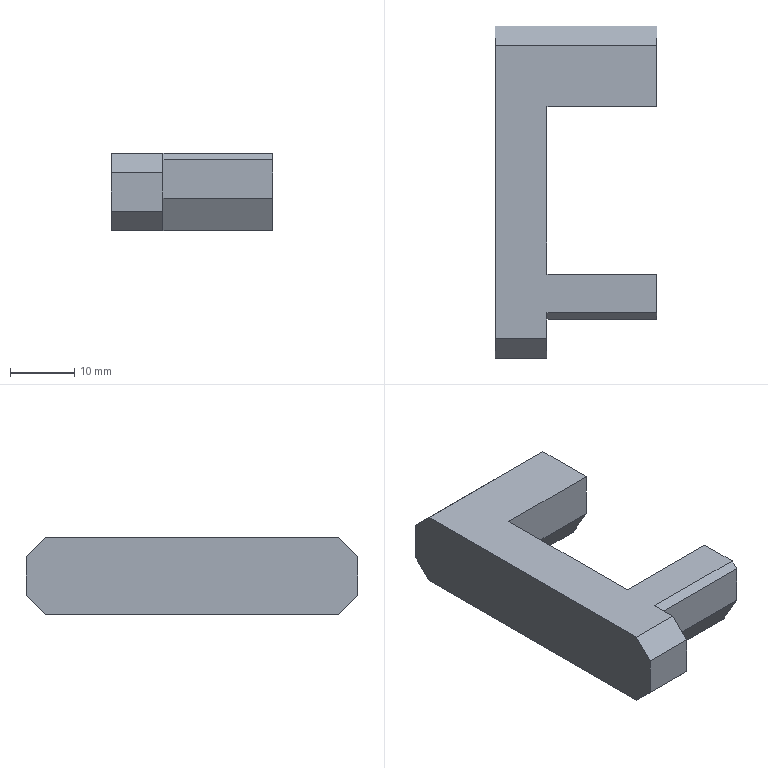Part | NX | features solid 2 | 1 solid | 19 faces | box 25 x 51.5 x 12 mm | volume 8371 mm3 | plane 19
STEP:
#1=CARTESIAN_POINT('',(256.5,-270.,46.5));
#2=VERTEX_POINT('',#1);
#3=CARTESIAN_POINT('',(256.5,-270.,52.5));
#4=VERTEX_POINT('',#3);
#5=CARTESIAN_POINT('',(256.5,-270.,46.5));
#6=DIRECTION('',(0.,0.,1.));
#7=VECTOR('',#6,1000.);
#8=LINE('',#5,#7);
#9=EDGE_CURVE('',#2,#4,#8,.T.);
#10=ORIENTED_EDGE('',*,*,#9,.F.);
#11=CARTESIAN_POINT('',(256.5,-267.113,41.5));
#12=VERTEX_POINT('',#11);
#13=CARTESIAN_POINT('',(256.5,-267.113,41.5));
#14=DIRECTION('',(0.,-0.5,0.866));
#15=VECTOR('',#14,1000.);
#16=LINE('',#13,#15);
#17=EDGE_CURVE('',#12,#2,#16,.T.);
#18=ORIENTED_EDGE('',*,*,#17,.F.);
#19=CARTESIAN_POINT('',(256.5,-263.,41.5));
#20=VERTEX_POINT('',#19);
#21=CARTESIAN_POINT('',(256.5,-263.,41.5));
#22=DIRECTION('',(0.,-1.,0.));
#23=VECTOR('',#22,1000.);
#24=LINE('',#21,#23);
#25=EDGE_CURVE('',#20,#12,#24,.T.);
#26=ORIENTED_EDGE('',*,*,#25,.F.);
#27=CARTESIAN_POINT('',(256.5,-263.,53.5));
#28=VERTEX_POINT('',#27);
#29=CARTESIAN_POINT('',(256.5,-263.,41.5));
#30=DIRECTION('',(0.,0.,1.));
#31=VECTOR('',#30,1000.);
#32=LINE('',#29,#31);
#33=EDGE_CURVE('',#20,#28,#32,.T.);
#34=ORIENTED_EDGE('',*,*,#33,.T.);
#35=CARTESIAN_POINT('',(256.5,-269.,53.5));
#36=VERTEX_POINT('',#35);
#37=CARTESIAN_POINT('',(256.5,-269.,53.5));
#38=DIRECTION('',(0.,1.,0.));
#39=VECTOR('',#38,1000.);
#40=LINE('',#37,#39);
#41=EDGE_CURVE('',#36,#28,#40,.T.);
#42=ORIENTED_EDGE('',*,*,#41,.F.);
#43=CARTESIAN_POINT('',(256.5,-269.,53.5));
#44=DIRECTION('',(0.,-0.7071,-0.7071));
#45=VECTOR('',#44,1000.);
#46=LINE('',#43,#45);
#47=EDGE_CURVE('',#36,#4,#46,.T.);
#48=ORIENTED_EDGE('',*,*,#47,.T.);
#49=EDGE_LOOP('',(#10,#18,#26,#34,#42,#48));
#50=FACE_BOUND('',#49,.T.);
#51=CARTESIAN_POINT('',(256.5,-276.,53.5));
#52=DIRECTION('',(-1.,0.,0.));
#53=DIRECTION('',(0.,0.,1.));
#54=AXIS2_PLACEMENT_3D('',#51,#52,#53);
#55=PLANE('',#54);
#56=ADVANCED_FACE('',(#50),#55,.F.);
#57=CARTESIAN_POINT('',(256.5,-237.,53.5));
#58=VERTEX_POINT('',#57);
#59=CARTESIAN_POINT('',(256.5,-227.5,53.5));
#60=VERTEX_POINT('',#59);
#61=CARTESIAN_POINT('',(256.5,-237.,53.5));
#62=DIRECTION('',(0.,1.,0.));
#63=VECTOR('',#62,1000.);
#64=LINE('',#61,#63);
#65=EDGE_CURVE('',#58,#60,#64,.T.);
#66=ORIENTED_EDGE('',*,*,#65,.F.);
#67=CARTESIAN_POINT('',(256.5,-237.,46.5));
#68=VERTEX_POINT('',#67);
#69=CARTESIAN_POINT('',(256.5,-237.,53.5));
#70=DIRECTION('',(0.,0.,-1.));
#71=VECTOR('',#70,1000.);
#72=LINE('',#69,#71);
#73=EDGE_CURVE('',#58,#68,#72,.T.);
#74=ORIENTED_EDGE('',*,*,#73,.T.);
#75=CARTESIAN_POINT('',(256.5,-234.113,41.5));
#76=VERTEX_POINT('',#75);
#77=CARTESIAN_POINT('',(256.5,-234.113,41.5));
#78=DIRECTION('',(0.,-0.5,0.866));
#79=VECTOR('',#78,1000.);
#80=LINE('',#77,#79);
#81=EDGE_CURVE('',#76,#68,#80,.T.);
#82=ORIENTED_EDGE('',*,*,#81,.F.);
#83=CARTESIAN_POINT('',(256.5,-227.5,41.5));
#84=VERTEX_POINT('',#83);
#85=CARTESIAN_POINT('',(256.5,-227.5,41.5));
#86=DIRECTION('',(0.,-1.,0.));
#87=VECTOR('',#86,1000.);
#88=LINE('',#85,#87);
#89=EDGE_CURVE('',#84,#76,#88,.T.);
#90=ORIENTED_EDGE('',*,*,#89,.F.);
#91=CARTESIAN_POINT('',(256.5,-224.5,44.5));
#92=VERTEX_POINT('',#91);
#93=CARTESIAN_POINT('',(256.5,-227.5,41.5));
#94=DIRECTION('',(0.,0.7071,0.7071));
#95=VECTOR('',#94,1000.);
#96=LINE('',#93,#95);
#97=EDGE_CURVE('',#84,#92,#96,.T.);
#98=ORIENTED_EDGE('',*,*,#97,.T.);
#99=CARTESIAN_POINT('',(256.5,-224.5,50.5));
#100=VERTEX_POINT('',#99);
#101=CARTESIAN_POINT('',(256.5,-224.5,50.5));
#102=DIRECTION('',(0.,0.,-1.));
#103=VECTOR('',#102,1000.);
#104=LINE('',#101,#103);
#105=EDGE_CURVE('',#100,#92,#104,.T.);
#106=ORIENTED_EDGE('',*,*,#105,.F.);
#107=CARTESIAN_POINT('',(256.5,-224.5,50.5));
#108=DIRECTION('',(0.,-0.7071,0.7071));
#109=VECTOR('',#108,1000.);
#110=LINE('',#107,#109);
#111=EDGE_CURVE('',#100,#60,#110,.T.);
#112=ORIENTED_EDGE('',*,*,#111,.T.);
#113=EDGE_LOOP('',(#66,#74,#82,#90,#98,#106,#112));
#114=FACE_BOUND('',#113,.T.);
#115=CARTESIAN_POINT('',(256.5,-276.,53.5));
#116=DIRECTION('',(-1.,0.,0.));
#117=DIRECTION('',(0.,0.,1.));
#118=AXIS2_PLACEMENT_3D('',#115,#116,#117);
#119=PLANE('',#118);
#120=ADVANCED_FACE('',(#114),#119,.F.);
#121=CARTESIAN_POINT('',(239.5,-269.,53.5));
#122=VERTEX_POINT('',#121);
#123=CARTESIAN_POINT('',(239.5,-269.,53.5));
#124=DIRECTION('',(1.,0.,0.));
#125=VECTOR('',#124,1000.);
#126=LINE('',#123,#125);
#127=EDGE_CURVE('',#122,#36,#126,.T.);
#128=ORIENTED_EDGE('',*,*,#127,.F.);
#129=CARTESIAN_POINT('',(239.5,-270.,52.5));
#130=VERTEX_POINT('',#129);
#131=CARTESIAN_POINT('',(239.5,-270.,52.5));
#132=DIRECTION('',(0.,0.7071,0.7071));
#133=VECTOR('',#132,1000.);
#134=LINE('',#131,#133);
#135=EDGE_CURVE('',#130,#122,#134,.T.);
#136=ORIENTED_EDGE('',*,*,#135,.F.);
#137=CARTESIAN_POINT('',(239.5,-270.,52.5));
#138=DIRECTION('',(1.,0.,0.));
#139=VECTOR('',#138,1000.);
#140=LINE('',#137,#139);
#141=EDGE_CURVE('',#130,#4,#140,.T.);
#142=ORIENTED_EDGE('',*,*,#141,.T.);
#143=ORIENTED_EDGE('',*,*,#47,.F.);
#144=EDGE_LOOP('',(#128,#136,#142,#143));
#145=FACE_BOUND('',#144,.T.);
#146=CARTESIAN_POINT('',(248.,-269.5,53.));
#147=DIRECTION('',(0.,-0.7071,0.7071));
#148=DIRECTION('',(0.,-0.7071,-0.7071));
#149=AXIS2_PLACEMENT_3D('',#146,#147,#148);
#150=PLANE('',#149);
#151=ADVANCED_FACE('',(#145),#150,.T.);
#152=CARTESIAN_POINT('',(239.5,-270.,46.5));
#153=VERTEX_POINT('',#152);
#154=CARTESIAN_POINT('',(239.5,-270.,46.5));
#155=DIRECTION('',(0.,0.,1.));
#156=VECTOR('',#155,1000.);
#157=LINE('',#154,#156);
#158=EDGE_CURVE('',#153,#130,#157,.T.);
#159=ORIENTED_EDGE('',*,*,#158,.F.);
#160=CARTESIAN_POINT('',(256.5,-270.,46.5));
#161=DIRECTION('',(-1.,0.,0.));
#162=VECTOR('',#161,1000.);
#163=LINE('',#160,#162);
#164=EDGE_CURVE('',#2,#153,#163,.T.);
#165=ORIENTED_EDGE('',*,*,#164,.F.);
#166=ORIENTED_EDGE('',*,*,#9,.T.);
#167=ORIENTED_EDGE('',*,*,#141,.F.);
#168=EDGE_LOOP('',(#159,#165,#166,#167));
#169=FACE_BOUND('',#168,.T.);
#170=CARTESIAN_POINT('',(256.5,-270.,46.5));
#171=DIRECTION('',(0.,1.,0.));
#172=DIRECTION('',(0.,0.,1.));
#173=AXIS2_PLACEMENT_3D('',#170,#171,#172);
#174=PLANE('',#173);
#175=ADVANCED_FACE('',(#169),#174,.F.);
#176=ORIENTED_EDGE('',*,*,#164,.T.);
#177=CARTESIAN_POINT('',(239.5,-267.113,41.5));
#178=VERTEX_POINT('',#177);
#179=CARTESIAN_POINT('',(239.5,-267.113,41.5));
#180=DIRECTION('',(0.,-0.5,0.866));
#181=VECTOR('',#180,1000.);
#182=LINE('',#179,#181);
#183=EDGE_CURVE('',#178,#153,#182,.T.);
#184=ORIENTED_EDGE('',*,*,#183,.F.);
#185=CARTESIAN_POINT('',(256.5,-267.113,41.5));
#186=DIRECTION('',(-1.,0.,0.));
#187=VECTOR('',#186,1000.);
#188=LINE('',#185,#187);
#189=EDGE_CURVE('',#12,#178,#188,.T.);
#190=ORIENTED_EDGE('',*,*,#189,.F.);
#191=ORIENTED_EDGE('',*,*,#17,.T.);
#192=EDGE_LOOP('',(#176,#184,#190,#191));
#193=FACE_BOUND('',#192,.T.);
#194=CARTESIAN_POINT('',(256.5,-267.113,41.5));
#195=DIRECTION('',(0.,0.866,0.5));
#196=DIRECTION('',(0.,-0.5,0.866));
#197=AXIS2_PLACEMENT_3D('',#194,#195,#196);
#198=PLANE('',#197);
#199=ADVANCED_FACE('',(#193),#198,.F.);
#200=ORIENTED_EDGE('',*,*,#89,.T.);
#201=CARTESIAN_POINT('',(239.5,-234.113,41.5));
#202=VERTEX_POINT('',#201);
#203=CARTESIAN_POINT('',(256.5,-234.113,41.5));
#204=DIRECTION('',(-1.,0.,0.));
#205=VECTOR('',#204,1000.);
#206=LINE('',#203,#205);
#207=EDGE_CURVE('',#76,#202,#206,.T.);
#208=ORIENTED_EDGE('',*,*,#207,.T.);
#209=CARTESIAN_POINT('',(239.5,-263.,41.5));
#210=VERTEX_POINT('',#209);
#211=CARTESIAN_POINT('',(239.5,-263.,41.5));
#212=DIRECTION('',(0.,1.,0.));
#213=VECTOR('',#212,1000.);
#214=LINE('',#211,#213);
#215=EDGE_CURVE('',#210,#202,#214,.T.);
#216=ORIENTED_EDGE('',*,*,#215,.F.);
#217=CARTESIAN_POINT('',(256.5,-263.,41.5));
#218=DIRECTION('',(-1.,0.,0.));
#219=VECTOR('',#218,1000.);
#220=LINE('',#217,#219);
#221=EDGE_CURVE('',#20,#210,#220,.T.);
#222=ORIENTED_EDGE('',*,*,#221,.F.);
#223=ORIENTED_EDGE('',*,*,#25,.T.);
#224=ORIENTED_EDGE('',*,*,#189,.T.);
#225=CARTESIAN_POINT('',(239.5,-273.,41.5));
#226=VERTEX_POINT('',#225);
#227=CARTESIAN_POINT('',(239.5,-273.,41.5));
#228=DIRECTION('',(0.,1.,0.));
#229=VECTOR('',#228,1000.);
#230=LINE('',#227,#229);
#231=EDGE_CURVE('',#226,#178,#230,.T.);
#232=ORIENTED_EDGE('',*,*,#231,.F.);
#233=CARTESIAN_POINT('',(231.5,-273.,41.5));
#234=VERTEX_POINT('',#233);
#235=CARTESIAN_POINT('',(231.5,-273.,41.5));
#236=DIRECTION('',(1.,0.,0.));
#237=VECTOR('',#236,1000.);
#238=LINE('',#235,#237);
#239=EDGE_CURVE('',#234,#226,#238,.T.);
#240=ORIENTED_EDGE('',*,*,#239,.F.);
#241=CARTESIAN_POINT('',(231.5,-227.5,41.5));
#242=VERTEX_POINT('',#241);
#243=CARTESIAN_POINT('',(231.5,-227.5,41.5));
#244=DIRECTION('',(0.,-1.,0.));
#245=VECTOR('',#244,1000.);
#246=LINE('',#243,#245);
#247=EDGE_CURVE('',#242,#234,#246,.T.);
#248=ORIENTED_EDGE('',*,*,#247,.F.);
#249=CARTESIAN_POINT('',(231.5,-227.5,41.5));
#250=DIRECTION('',(1.,0.,0.));
#251=VECTOR('',#250,1000.);
#252=LINE('',#249,#251);
#253=EDGE_CURVE('',#242,#84,#252,.T.);
#254=ORIENTED_EDGE('',*,*,#253,.T.);
#255=EDGE_LOOP('',(#200,#208,#216,#222,#223,#224,#232,#240,#248,#254));
#256=FACE_BOUND('',#255,.T.);
#257=CARTESIAN_POINT('',(256.5,-224.5,41.5));
#258=DIRECTION('',(0.,0.,-1.));
#259=DIRECTION('',(0.,1.,0.));
#260=AXIS2_PLACEMENT_3D('',#257,#258,#259);
#261=PLANE('',#260);
#262=ADVANCED_FACE('',(#256),#261,.T.);
#263=ORIENTED_EDGE('',*,*,#253,.F.);
#264=CARTESIAN_POINT('',(231.5,-224.5,44.5));
#265=VERTEX_POINT('',#264);
#266=CARTESIAN_POINT('',(231.5,-224.5,44.5));
#267=DIRECTION('',(0.,-0.7071,-0.7071));
#268=VECTOR('',#267,1000.);
#269=LINE('',#266,#268);
#270=EDGE_CURVE('',#265,#242,#269,.T.);
#271=ORIENTED_EDGE('',*,*,#270,.F.);
#272=CARTESIAN_POINT('',(231.5,-224.5,44.5));
#273=DIRECTION('',(1.,0.,0.));
#274=VECTOR('',#273,1000.);
#275=LINE('',#272,#274);
#276=EDGE_CURVE('',#265,#92,#275,.T.);
#277=ORIENTED_EDGE('',*,*,#276,.T.);
#278=ORIENTED_EDGE('',*,*,#97,.F.);
#279=EDGE_LOOP('',(#263,#271,#277,#278));
#280=FACE_BOUND('',#279,.T.);
#281=CARTESIAN_POINT('',(244.,-226.,43.));
#282=DIRECTION('',(0.,0.7071,-0.7071));
#283=DIRECTION('',(0.,0.7071,0.7071));
#284=AXIS2_PLACEMENT_3D('',#281,#282,#283);
#285=PLANE('',#284);
#286=ADVANCED_FACE('',(#280),#285,.T.);
#287=ORIENTED_EDGE('',*,*,#105,.T.);
#288=ORIENTED_EDGE('',*,*,#276,.F.);
#289=CARTESIAN_POINT('',(231.5,-224.5,50.5));
#290=VERTEX_POINT('',#289);
#291=CARTESIAN_POINT('',(231.5,-224.5,50.5));
#292=DIRECTION('',(0.,0.,-1.));
#293=VECTOR('',#292,1000.);
#294=LINE('',#291,#293);
#295=EDGE_CURVE('',#290,#265,#294,.T.);
#296=ORIENTED_EDGE('',*,*,#295,.F.);
#297=CARTESIAN_POINT('',(231.5,-224.5,50.5));
#298=DIRECTION('',(1.,0.,0.));
#299=VECTOR('',#298,1000.);
#300=LINE('',#297,#299);
#301=EDGE_CURVE('',#290,#100,#300,.T.);
#302=ORIENTED_EDGE('',*,*,#301,.T.);
#303=EDGE_LOOP('',(#287,#288,#296,#302));
#304=FACE_BOUND('',#303,.T.);
#305=CARTESIAN_POINT('',(256.5,-224.5,53.5));
#306=DIRECTION('',(0.,1.,0.));
#307=DIRECTION('',(0.,0.,1.));
#308=AXIS2_PLACEMENT_3D('',#305,#306,#307);
#309=PLANE('',#308);
#310=ADVANCED_FACE('',(#304),#309,.T.);
#311=ORIENTED_EDGE('',*,*,#301,.F.);
#312=CARTESIAN_POINT('',(231.5,-227.5,53.5));
#313=VERTEX_POINT('',#312);
#314=CARTESIAN_POINT('',(231.5,-227.5,53.5));
#315=DIRECTION('',(0.,0.7071,-0.7071));
#316=VECTOR('',#315,1000.);
#317=LINE('',#314,#316);
#318=EDGE_CURVE('',#313,#290,#317,.T.);
#319=ORIENTED_EDGE('',*,*,#318,.F.);
#320=CARTESIAN_POINT('',(231.5,-227.5,53.5));
#321=DIRECTION('',(1.,0.,0.));
#322=VECTOR('',#321,1000.);
#323=LINE('',#320,#322);
#324=EDGE_CURVE('',#313,#60,#323,.T.);
#325=ORIENTED_EDGE('',*,*,#324,.T.);
#326=ORIENTED_EDGE('',*,*,#111,.F.);
#327=EDGE_LOOP('',(#311,#319,#325,#326));
#328=FACE_BOUND('',#327,.T.);
#329=CARTESIAN_POINT('',(244.,-226.,52.));
#330=DIRECTION('',(0.,0.7071,0.7071));
#331=DIRECTION('',(0.,-0.7071,0.7071));
#332=AXIS2_PLACEMENT_3D('',#329,#330,#331);
#333=PLANE('',#332);
#334=ADVANCED_FACE('',(#328),#333,.T.);
#335=CARTESIAN_POINT('',(231.5,-273.,53.5));
#336=VERTEX_POINT('',#335);
#337=CARTESIAN_POINT('',(231.5,-273.,53.5));
#338=DIRECTION('',(0.,1.,0.));
#339=VECTOR('',#338,1000.);
#340=LINE('',#337,#339);
#341=EDGE_CURVE('',#336,#313,#340,.T.);
#342=ORIENTED_EDGE('',*,*,#341,.F.);
#343=CARTESIAN_POINT('',(239.5,-273.,53.5));
#344=VERTEX_POINT('',#343);
#345=CARTESIAN_POINT('',(231.5,-273.,53.5));
#346=DIRECTION('',(1.,0.,0.));
#347=VECTOR('',#346,1000.);
#348=LINE('',#345,#347);
#349=EDGE_CURVE('',#336,#344,#348,.T.);
#350=ORIENTED_EDGE('',*,*,#349,.T.);
#351=CARTESIAN_POINT('',(239.5,-273.,53.5));
#352=DIRECTION('',(0.,1.,0.));
#353=VECTOR('',#352,1000.);
#354=LINE('',#351,#353);
#355=EDGE_CURVE('',#344,#122,#354,.T.);
#356=ORIENTED_EDGE('',*,*,#355,.T.);
#357=ORIENTED_EDGE('',*,*,#127,.T.);
#358=ORIENTED_EDGE('',*,*,#41,.T.);
#359=CARTESIAN_POINT('',(239.5,-263.,53.5));
#360=VERTEX_POINT('',#359);
#361=CARTESIAN_POINT('',(256.5,-263.,53.5));
#362=DIRECTION('',(-1.,0.,0.));
#363=VECTOR('',#362,1000.);
#364=LINE('',#361,#363);
#365=EDGE_CURVE('',#28,#360,#364,.T.);
#366=ORIENTED_EDGE('',*,*,#365,.T.);
#367=CARTESIAN_POINT('',(239.5,-237.,53.5));
#368=VERTEX_POINT('',#367);
#369=CARTESIAN_POINT('',(239.5,-263.,53.5));
#370=DIRECTION('',(0.,1.,0.));
#371=VECTOR('',#370,1000.);
#372=LINE('',#369,#371);
#373=EDGE_CURVE('',#360,#368,#372,.T.);
#374=ORIENTED_EDGE('',*,*,#373,.T.);
#375=CARTESIAN_POINT('',(256.5,-237.,53.5));
#376=DIRECTION('',(-1.,0.,0.));
#377=VECTOR('',#376,1000.);
#378=LINE('',#375,#377);
#379=EDGE_CURVE('',#58,#368,#378,.T.);
#380=ORIENTED_EDGE('',*,*,#379,.F.);
#381=ORIENTED_EDGE('',*,*,#65,.T.);
#382=ORIENTED_EDGE('',*,*,#324,.F.);
#383=EDGE_LOOP('',(#342,#350,#356,#357,#358,#366,#374,#380,#381,#382));
#384=FACE_BOUND('',#383,.T.);
#385=CARTESIAN_POINT('',(256.5,-276.,53.5));
#386=DIRECTION('',(0.,0.,1.));
#387=DIRECTION('',(0.,-1.,0.));
#388=AXIS2_PLACEMENT_3D('',#385,#386,#387);
#389=PLANE('',#388);
#390=ADVANCED_FACE('',(#384),#389,.T.);
#391=ORIENTED_EDGE('',*,*,#379,.T.);
#392=CARTESIAN_POINT('',(239.5,-237.,46.5));
#393=VERTEX_POINT('',#392);
#394=CARTESIAN_POINT('',(239.5,-237.,46.5));
#395=DIRECTION('',(0.,0.,1.));
#396=VECTOR('',#395,1000.);
#397=LINE('',#394,#396);
#398=EDGE_CURVE('',#393,#368,#397,.T.);
#399=ORIENTED_EDGE('',*,*,#398,.F.);
#400=CARTESIAN_POINT('',(256.5,-237.,46.5));
#401=DIRECTION('',(-1.,0.,0.));
#402=VECTOR('',#401,1000.);
#403=LINE('',#400,#402);
#404=EDGE_CURVE('',#68,#393,#403,.T.);
#405=ORIENTED_EDGE('',*,*,#404,.F.);
#406=ORIENTED_EDGE('',*,*,#73,.F.);
#407=EDGE_LOOP('',(#391,#399,#405,#406));
#408=FACE_BOUND('',#407,.T.);
#409=CARTESIAN_POINT('',(256.5,-237.,46.5));
#410=DIRECTION('',(0.,1.,0.));
#411=DIRECTION('',(0.,0.,1.));
#412=AXIS2_PLACEMENT_3D('',#409,#410,#411);
#413=PLANE('',#412);
#414=ADVANCED_FACE('',(#408),#413,.F.);
#415=ORIENTED_EDGE('',*,*,#404,.T.);
#416=CARTESIAN_POINT('',(239.5,-234.113,41.5));
#417=DIRECTION('',(0.,-0.5,0.866));
#418=VECTOR('',#417,1000.);
#419=LINE('',#416,#418);
#420=EDGE_CURVE('',#202,#393,#419,.T.);
#421=ORIENTED_EDGE('',*,*,#420,.F.);
#422=ORIENTED_EDGE('',*,*,#207,.F.);
#423=ORIENTED_EDGE('',*,*,#81,.T.);
#424=EDGE_LOOP('',(#415,#421,#422,#423));
#425=FACE_BOUND('',#424,.T.);
#426=CARTESIAN_POINT('',(256.5,-234.113,41.5));
#427=DIRECTION('',(0.,0.866,0.5));
#428=DIRECTION('',(0.,-0.5,0.866));
#429=AXIS2_PLACEMENT_3D('',#426,#427,#428);
#430=PLANE('',#429);
#431=ADVANCED_FACE('',(#425),#430,.F.);
#432=CARTESIAN_POINT('',(239.5,-263.,53.5));
#433=DIRECTION('',(0.,0.,-1.));
#434=VECTOR('',#433,1000.);
#435=LINE('',#432,#434);
#436=EDGE_CURVE('',#360,#210,#435,.T.);
#437=ORIENTED_EDGE('',*,*,#436,.T.);
#438=ORIENTED_EDGE('',*,*,#215,.T.);
#439=ORIENTED_EDGE('',*,*,#420,.T.);
#440=ORIENTED_EDGE('',*,*,#398,.T.);
#441=ORIENTED_EDGE('',*,*,#373,.F.);
#442=EDGE_LOOP('',(#437,#438,#439,#440,#441));
#443=FACE_BOUND('',#442,.T.);
#444=CARTESIAN_POINT('',(239.5,-276.,53.5));
#445=DIRECTION('',(1.,0.,0.));
#446=DIRECTION('',(0.,0.,-1.));
#447=AXIS2_PLACEMENT_3D('',#444,#445,#446);
#448=PLANE('',#447);
#449=ADVANCED_FACE('',(#443),#448,.T.);
#450=ORIENTED_EDGE('',*,*,#231,.T.);
#451=ORIENTED_EDGE('',*,*,#183,.T.);
#452=ORIENTED_EDGE('',*,*,#158,.T.);
#453=ORIENTED_EDGE('',*,*,#135,.T.);
#454=ORIENTED_EDGE('',*,*,#355,.F.);
#455=CARTESIAN_POINT('',(239.5,-276.,50.5));
#456=VERTEX_POINT('',#455);
#457=CARTESIAN_POINT('',(239.5,-273.,53.5));
#458=DIRECTION('',(0.,-0.7071,-0.7071));
#459=VECTOR('',#458,1000.);
#460=LINE('',#457,#459);
#461=EDGE_CURVE('',#344,#456,#460,.T.);
#462=ORIENTED_EDGE('',*,*,#461,.T.);
#463=CARTESIAN_POINT('',(239.5,-276.,44.5));
#464=VERTEX_POINT('',#463);
#465=CARTESIAN_POINT('',(239.5,-276.,44.5));
#466=DIRECTION('',(0.,0.,1.));
#467=VECTOR('',#466,1000.);
#468=LINE('',#465,#467);
#469=EDGE_CURVE('',#464,#456,#468,.T.);
#470=ORIENTED_EDGE('',*,*,#469,.F.);
#471=CARTESIAN_POINT('',(239.5,-276.,44.5));
#472=DIRECTION('',(0.,0.7071,-0.7071));
#473=VECTOR('',#472,1000.);
#474=LINE('',#471,#473);
#475=EDGE_CURVE('',#464,#226,#474,.T.);
#476=ORIENTED_EDGE('',*,*,#475,.T.);
#477=EDGE_LOOP('',(#450,#451,#452,#453,#454,#462,#470,#476));
#478=FACE_BOUND('',#477,.T.);
#479=CARTESIAN_POINT('',(239.5,-276.,53.5));
#480=DIRECTION('',(1.,0.,0.));
#481=DIRECTION('',(0.,0.,-1.));
#482=AXIS2_PLACEMENT_3D('',#479,#480,#481);
#483=PLANE('',#482);
#484=ADVANCED_FACE('',(#478),#483,.T.);
#485=ORIENTED_EDGE('',*,*,#221,.T.);
#486=ORIENTED_EDGE('',*,*,#436,.F.);
#487=ORIENTED_EDGE('',*,*,#365,.F.);
#488=ORIENTED_EDGE('',*,*,#33,.F.);
#489=EDGE_LOOP('',(#485,#486,#487,#488));
#490=FACE_BOUND('',#489,.T.);
#491=CARTESIAN_POINT('',(256.5,-263.,53.5));
#492=DIRECTION('',(0.,-1.,0.));
#493=DIRECTION('',(0.,0.,-1.));
#494=AXIS2_PLACEMENT_3D('',#491,#492,#493);
#495=PLANE('',#494);
#496=ADVANCED_FACE('',(#490),#495,.F.);
#497=CARTESIAN_POINT('',(231.5,-276.,44.5));
#498=VERTEX_POINT('',#497);
#499=CARTESIAN_POINT('',(231.5,-276.,44.5));
#500=DIRECTION('',(1.,0.,0.));
#501=VECTOR('',#500,1000.);
#502=LINE('',#499,#501);
#503=EDGE_CURVE('',#498,#464,#502,.T.);
#504=ORIENTED_EDGE('',*,*,#503,.F.);
#505=CARTESIAN_POINT('',(231.5,-273.,41.5));
#506=DIRECTION('',(0.,-0.7071,0.7071));
#507=VECTOR('',#506,1000.);
#508=LINE('',#505,#507);
#509=EDGE_CURVE('',#234,#498,#508,.T.);
#510=ORIENTED_EDGE('',*,*,#509,.F.);
#511=ORIENTED_EDGE('',*,*,#239,.T.);
#512=ORIENTED_EDGE('',*,*,#475,.F.);
#513=EDGE_LOOP('',(#504,#510,#511,#512));
#514=FACE_BOUND('',#513,.T.);
#515=CARTESIAN_POINT('',(235.5,-274.5,43.));
#516=DIRECTION('',(0.,-0.7071,-0.7071));
#517=DIRECTION('',(0.,0.7071,-0.7071));
#518=AXIS2_PLACEMENT_3D('',#515,#516,#517);
#519=PLANE('',#518);
#520=ADVANCED_FACE('',(#514),#519,.T.);
#521=ORIENTED_EDGE('',*,*,#318,.T.);
#522=ORIENTED_EDGE('',*,*,#295,.T.);
#523=ORIENTED_EDGE('',*,*,#270,.T.);
#524=ORIENTED_EDGE('',*,*,#247,.T.);
#525=ORIENTED_EDGE('',*,*,#509,.T.);
#526=CARTESIAN_POINT('',(231.5,-276.,50.5));
#527=VERTEX_POINT('',#526);
#528=CARTESIAN_POINT('',(231.5,-276.,44.5));
#529=DIRECTION('',(0.,0.,1.));
#530=VECTOR('',#529,1000.);
#531=LINE('',#528,#530);
#532=EDGE_CURVE('',#498,#527,#531,.T.);
#533=ORIENTED_EDGE('',*,*,#532,.T.);
#534=CARTESIAN_POINT('',(231.5,-276.,50.5));
#535=DIRECTION('',(0.,0.7071,0.7071));
#536=VECTOR('',#535,1000.);
#537=LINE('',#534,#536);
#538=EDGE_CURVE('',#527,#336,#537,.T.);
#539=ORIENTED_EDGE('',*,*,#538,.T.);
#540=ORIENTED_EDGE('',*,*,#341,.T.);
#541=EDGE_LOOP('',(#521,#522,#523,#524,#525,#533,#539,#540));
#542=FACE_BOUND('',#541,.T.);
#543=CARTESIAN_POINT('',(231.5,-276.,53.5));
#544=DIRECTION('',(-1.,0.,0.));
#545=DIRECTION('',(0.,0.,1.));
#546=AXIS2_PLACEMENT_3D('',#543,#544,#545);
#547=PLANE('',#546);
#548=ADVANCED_FACE('',(#542),#547,.T.);
#549=ORIENTED_EDGE('',*,*,#349,.F.);
#550=ORIENTED_EDGE('',*,*,#538,.F.);
#551=CARTESIAN_POINT('',(231.5,-276.,50.5));
#552=DIRECTION('',(1.,0.,0.));
#553=VECTOR('',#552,1000.);
#554=LINE('',#551,#553);
#555=EDGE_CURVE('',#527,#456,#554,.T.);
#556=ORIENTED_EDGE('',*,*,#555,.T.);
#557=ORIENTED_EDGE('',*,*,#461,.F.);
#558=EDGE_LOOP('',(#549,#550,#556,#557));
#559=FACE_BOUND('',#558,.T.);
#560=CARTESIAN_POINT('',(235.5,-274.5,52.));
#561=DIRECTION('',(0.,-0.7071,0.7071));
#562=DIRECTION('',(0.,-0.7071,-0.7071));
#563=AXIS2_PLACEMENT_3D('',#560,#561,#562);
#564=PLANE('',#563);
#565=ADVANCED_FACE('',(#559),#564,.T.);
#566=ORIENTED_EDGE('',*,*,#469,.T.);
#567=ORIENTED_EDGE('',*,*,#555,.F.);
#568=ORIENTED_EDGE('',*,*,#532,.F.);
#569=ORIENTED_EDGE('',*,*,#503,.T.);
#570=EDGE_LOOP('',(#566,#567,#568,#569));
#571=FACE_BOUND('',#570,.T.);
#572=CARTESIAN_POINT('',(256.5,-276.,41.5));
#573=DIRECTION('',(0.,-1.,0.));
#574=DIRECTION('',(0.,0.,-1.));
#575=AXIS2_PLACEMENT_3D('',#572,#573,#574);
#576=PLANE('',#575);
#577=ADVANCED_FACE('',(#571),#576,.T.);
#578=CLOSED_SHELL('',(#56,#120,#151,#175,#199,#262,#286,#310,#334,#390,#414,#431,#449,#484,#496,#520,#548,#565,#577));
#579=MANIFOLD_SOLID_BREP('',#578);
#580=(LENGTH_UNIT()NAMED_UNIT(*)SI_UNIT(.MILLI.,.METRE.));
#581=UNCERTAINTY_MEASURE_WITH_UNIT(LENGTH_MEASURE(0.00001),#580,'','');
#582=(NAMED_UNIT(*)PLANE_ANGLE_UNIT()SI_UNIT($,.RADIAN.));
#583=(NAMED_UNIT(*)SI_UNIT($,.STERADIAN.)SOLID_ANGLE_UNIT());
#584=(GEOMETRIC_REPRESENTATION_CONTEXT(3)GLOBAL_UNCERTAINTY_ASSIGNED_CONTEXT((#581))GLOBAL_UNIT_ASSIGNED_CONTEXT((#580,#582,#583))REPRESENTATION_CONTEXT('',''));
#585=ADVANCED_BREP_SHAPE_REPRESENTATION('',(#579),#584);